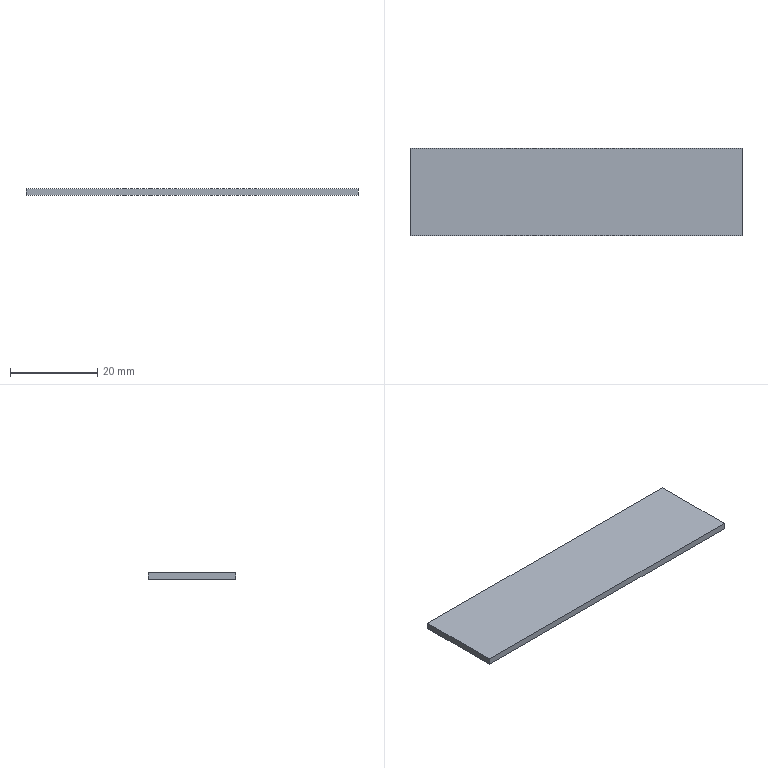Part | STEP file | FHD-021-008-01-C circuit breaker bracket 3 | 1 solid | 6 faces | box 76 x 20 x 1.5 mm | volume 2280 mm3 | plane 6
STEP:
#1=CARTESIAN_POINT('',(0.,0.,0.));
#2=DIRECTION('',(0.,0.,1.));
#3=DIRECTION('',(1.,0.,0.));
#4=AXIS2_PLACEMENT_3D('',#1,#2,#3);
#5=CARTESIAN_POINT('',(-38.,-10.,-1.5));
#6=VERTEX_POINT('',#5);
#7=CARTESIAN_POINT('',(-38.,10.,-1.5));
#8=VERTEX_POINT('',#7);
#9=CARTESIAN_POINT('',(-38.,0.,-1.5));
#10=DIRECTION('',(0.,1.,0.));
#11=VECTOR('',#10,1.);
#12=LINE('',#9,#11);
#13=CARTESIAN_POINT('',(0.,0.,-1.5));
#14=DIRECTION('',(0.,0.,-1.));
#15=DIRECTION('',(-1.,0.,0.));
#16=AXIS2_PLACEMENT_3D('',#13,#14,#15);
#17=PLANE('',#16);
#18=CARTESIAN_POINT('',(38.,0.));
#19=DIRECTION('',(0.,1.));
#20=VECTOR('',#19,1.);
#21=LINE('',#18,#20);
#22=(GEOMETRIC_REPRESENTATION_CONTEXT(2)PARAMETRIC_REPRESENTATION_CONTEXT()REPRESENTATION_CONTEXT('',''));
#23=DEFINITIONAL_REPRESENTATION('',(#21),#22);
#24=PCURVE('',#17,#23);
#25=CARTESIAN_POINT('',(-38.,-10.,-1.5));
#26=DIRECTION('',(-1.,0.,0.));
#27=DIRECTION('',(0.,0.,1.));
#28=AXIS2_PLACEMENT_3D('',#25,#26,#27);
#29=PLANE('',#28);
#30=CARTESIAN_POINT('',(0.,10.));
#31=DIRECTION('',(0.,1.));
#32=VECTOR('',#31,1.);
#33=LINE('',#30,#32);
#34=(GEOMETRIC_REPRESENTATION_CONTEXT(2)PARAMETRIC_REPRESENTATION_CONTEXT()REPRESENTATION_CONTEXT('',''));
#35=DEFINITIONAL_REPRESENTATION('',(#33),#34);
#36=PCURVE('',#29,#35);
#37=SURFACE_CURVE('',#12,(#24,#36),.PCURVE_S1.);
#38=EDGE_CURVE('',#6,#8,#37,.T.);
#39=ORIENTED_EDGE('',*,*,#38,.T.);
#40=CARTESIAN_POINT('',(38.,10.,-1.5));
#41=VERTEX_POINT('',#40);
#42=CARTESIAN_POINT('',(0.,10.,-1.5));
#43=DIRECTION('',(1.,0.,0.));
#44=VECTOR('',#43,1.);
#45=LINE('',#42,#44);
#46=CARTESIAN_POINT('',(0.,10.));
#47=DIRECTION('',(-1.,0.));
#48=VECTOR('',#47,1.);
#49=LINE('',#46,#48);
#50=(GEOMETRIC_REPRESENTATION_CONTEXT(2)PARAMETRIC_REPRESENTATION_CONTEXT()REPRESENTATION_CONTEXT('',''));
#51=DEFINITIONAL_REPRESENTATION('',(#49),#50);
#52=PCURVE('',#17,#51);
#53=CARTESIAN_POINT('',(-38.,10.,-1.5));
#54=DIRECTION('',(0.,1.,0.));
#55=DIRECTION('',(0.,0.,1.));
#56=AXIS2_PLACEMENT_3D('',#53,#54,#55);
#57=PLANE('',#56);
#58=CARTESIAN_POINT('',(0.,38.));
#59=DIRECTION('',(0.,1.));
#60=VECTOR('',#59,1.);
#61=LINE('',#58,#60);
#62=(GEOMETRIC_REPRESENTATION_CONTEXT(2)PARAMETRIC_REPRESENTATION_CONTEXT()REPRESENTATION_CONTEXT('',''));
#63=DEFINITIONAL_REPRESENTATION('',(#61),#62);
#64=PCURVE('',#57,#63);
#65=SURFACE_CURVE('',#45,(#52,#64),.PCURVE_S1.);
#66=EDGE_CURVE('',#8,#41,#65,.T.);
#67=ORIENTED_EDGE('',*,*,#66,.T.);
#68=CARTESIAN_POINT('',(38.,-10.,-1.5));
#69=VERTEX_POINT('',#68);
#70=CARTESIAN_POINT('',(38.,0.,-1.5));
#71=DIRECTION('',(0.,-1.,0.));
#72=VECTOR('',#71,1.);
#73=LINE('',#70,#72);
#74=CARTESIAN_POINT('',(-38.,0.));
#75=DIRECTION('',(0.,-1.));
#76=VECTOR('',#75,1.);
#77=LINE('',#74,#76);
#78=(GEOMETRIC_REPRESENTATION_CONTEXT(2)PARAMETRIC_REPRESENTATION_CONTEXT()REPRESENTATION_CONTEXT('',''));
#79=DEFINITIONAL_REPRESENTATION('',(#77),#78);
#80=PCURVE('',#17,#79);
#81=CARTESIAN_POINT('',(38.,-10.,-1.5));
#82=DIRECTION('',(1.,0.,0.));
#83=DIRECTION('',(0.,0.,-1.));
#84=AXIS2_PLACEMENT_3D('',#81,#82,#83);
#85=PLANE('',#84);
#86=CARTESIAN_POINT('',(0.,10.));
#87=DIRECTION('',(0.,-1.));
#88=VECTOR('',#87,1.);
#89=LINE('',#86,#88);
#90=(GEOMETRIC_REPRESENTATION_CONTEXT(2)PARAMETRIC_REPRESENTATION_CONTEXT()REPRESENTATION_CONTEXT('',''));
#91=DEFINITIONAL_REPRESENTATION('',(#89),#90);
#92=PCURVE('',#85,#91);
#93=SURFACE_CURVE('',#73,(#80,#92),.PCURVE_S1.);
#94=EDGE_CURVE('',#41,#69,#93,.T.);
#95=ORIENTED_EDGE('',*,*,#94,.T.);
#96=CARTESIAN_POINT('',(0.,-10.,-1.5));
#97=DIRECTION('',(-1.,0.,0.));
#98=VECTOR('',#97,1.);
#99=LINE('',#96,#98);
#100=CARTESIAN_POINT('',(0.,-10.));
#101=DIRECTION('',(1.,0.));
#102=VECTOR('',#101,1.);
#103=LINE('',#100,#102);
#104=(GEOMETRIC_REPRESENTATION_CONTEXT(2)PARAMETRIC_REPRESENTATION_CONTEXT()REPRESENTATION_CONTEXT('',''));
#105=DEFINITIONAL_REPRESENTATION('',(#103),#104);
#106=PCURVE('',#17,#105);
#107=CARTESIAN_POINT('',(-38.,-10.,-1.5));
#108=DIRECTION('',(0.,-1.,0.));
#109=DIRECTION('',(0.,0.,-1.));
#110=AXIS2_PLACEMENT_3D('',#107,#108,#109);
#111=PLANE('',#110);
#112=CARTESIAN_POINT('',(0.,38.));
#113=DIRECTION('',(0.,-1.));
#114=VECTOR('',#113,1.);
#115=LINE('',#112,#114);
#116=(GEOMETRIC_REPRESENTATION_CONTEXT(2)PARAMETRIC_REPRESENTATION_CONTEXT()REPRESENTATION_CONTEXT('',''));
#117=DEFINITIONAL_REPRESENTATION('',(#115),#116);
#118=PCURVE('',#111,#117);
#119=SURFACE_CURVE('',#99,(#106,#118),.PCURVE_S1.);
#120=EDGE_CURVE('',#69,#6,#119,.T.);
#121=ORIENTED_EDGE('',*,*,#120,.T.);
#122=EDGE_LOOP('',(#39,#67,#95,#121));
#123=FACE_BOUND('',#122,.T.);
#124=ADVANCED_FACE('',(#123),#17,.T.);
#125=ORIENTED_EDGE('',*,*,#66,.F.);
#126=CARTESIAN_POINT('',(-38.,10.,0.));
#127=VERTEX_POINT('',#126);
#128=CARTESIAN_POINT('',(-38.,10.,-1.5));
#129=DIRECTION('',(0.,0.,1.));
#130=VECTOR('',#129,1.);
#131=LINE('',#128,#130);
#132=CARTESIAN_POINT('',(0.,0.));
#133=DIRECTION('',(1.,0.));
#134=VECTOR('',#133,1.);
#135=LINE('',#132,#134);
#136=(GEOMETRIC_REPRESENTATION_CONTEXT(2)PARAMETRIC_REPRESENTATION_CONTEXT()REPRESENTATION_CONTEXT('',''));
#137=DEFINITIONAL_REPRESENTATION('',(#135),#136);
#138=PCURVE('',#57,#137);
#139=CARTESIAN_POINT('',(0.,20.));
#140=DIRECTION('',(1.,0.));
#141=VECTOR('',#140,1.);
#142=LINE('',#139,#141);
#143=(GEOMETRIC_REPRESENTATION_CONTEXT(2)PARAMETRIC_REPRESENTATION_CONTEXT()REPRESENTATION_CONTEXT('',''));
#144=DEFINITIONAL_REPRESENTATION('',(#142),#143);
#145=PCURVE('',#29,#144);
#146=SURFACE_CURVE('',#131,(#138,#145),.PCURVE_S1.);
#147=EDGE_CURVE('',#8,#127,#146,.T.);
#148=ORIENTED_EDGE('',*,*,#147,.T.);
#149=CARTESIAN_POINT('',(38.,10.,0.));
#150=VERTEX_POINT('',#149);
#151=CARTESIAN_POINT('',(-38.,10.,0.));
#152=DIRECTION('',(1.,0.,0.));
#153=VECTOR('',#152,1.);
#154=LINE('',#151,#153);
#155=CARTESIAN_POINT('',(1.5,0.));
#156=DIRECTION('',(0.,1.));
#157=VECTOR('',#156,1.);
#158=LINE('',#155,#157);
#159=(GEOMETRIC_REPRESENTATION_CONTEXT(2)PARAMETRIC_REPRESENTATION_CONTEXT()REPRESENTATION_CONTEXT('',''));
#160=DEFINITIONAL_REPRESENTATION('',(#158),#159);
#161=PCURVE('',#57,#160);
#162=CARTESIAN_POINT('',(0.,0.,0.));
#163=DIRECTION('',(0.,0.,-1.));
#164=DIRECTION('',(-1.,0.,0.));
#165=AXIS2_PLACEMENT_3D('',#162,#163,#164);
#166=PLANE('',#165);
#167=CARTESIAN_POINT('',(38.,10.));
#168=DIRECTION('',(-1.,0.));
#169=VECTOR('',#168,1.);
#170=LINE('',#167,#169);
#171=(GEOMETRIC_REPRESENTATION_CONTEXT(2)PARAMETRIC_REPRESENTATION_CONTEXT()REPRESENTATION_CONTEXT('',''));
#172=DEFINITIONAL_REPRESENTATION('',(#170),#171);
#173=PCURVE('',#166,#172);
#174=SURFACE_CURVE('',#154,(#161,#173),.PCURVE_S1.);
#175=EDGE_CURVE('',#127,#150,#174,.T.);
#176=ORIENTED_EDGE('',*,*,#175,.T.);
#177=CARTESIAN_POINT('',(38.,10.,-1.5));
#178=DIRECTION('',(0.,0.,-1.));
#179=VECTOR('',#178,1.);
#180=LINE('',#177,#179);
#181=CARTESIAN_POINT('',(0.,76.));
#182=DIRECTION('',(-1.,0.));
#183=VECTOR('',#182,1.);
#184=LINE('',#181,#183);
#185=(GEOMETRIC_REPRESENTATION_CONTEXT(2)PARAMETRIC_REPRESENTATION_CONTEXT()REPRESENTATION_CONTEXT('',''));
#186=DEFINITIONAL_REPRESENTATION('',(#184),#185);
#187=PCURVE('',#57,#186);
#188=CARTESIAN_POINT('',(0.,20.));
#189=DIRECTION('',(1.,0.));
#190=VECTOR('',#189,1.);
#191=LINE('',#188,#190);
#192=(GEOMETRIC_REPRESENTATION_CONTEXT(2)PARAMETRIC_REPRESENTATION_CONTEXT()REPRESENTATION_CONTEXT('',''));
#193=DEFINITIONAL_REPRESENTATION('',(#191),#192);
#194=PCURVE('',#85,#193);
#195=SURFACE_CURVE('',#180,(#187,#194),.PCURVE_S1.);
#196=EDGE_CURVE('',#150,#41,#195,.T.);
#197=ORIENTED_EDGE('',*,*,#196,.T.);
#198=EDGE_LOOP('',(#125,#148,#176,#197));
#199=FACE_BOUND('',#198,.T.);
#200=ADVANCED_FACE('',(#199),#57,.T.);
#201=ORIENTED_EDGE('',*,*,#38,.F.);
#202=CARTESIAN_POINT('',(-38.,-10.,0.));
#203=VERTEX_POINT('',#202);
#204=CARTESIAN_POINT('',(-38.,-10.,-1.5));
#205=DIRECTION('',(0.,0.,1.));
#206=VECTOR('',#205,1.);
#207=LINE('',#204,#206);
#208=CARTESIAN_POINT('',(0.,0.));
#209=DIRECTION('',(1.,0.));
#210=VECTOR('',#209,1.);
#211=LINE('',#208,#210);
#212=(GEOMETRIC_REPRESENTATION_CONTEXT(2)PARAMETRIC_REPRESENTATION_CONTEXT()REPRESENTATION_CONTEXT('',''));
#213=DEFINITIONAL_REPRESENTATION('',(#211),#212);
#214=PCURVE('',#29,#213);
#215=CARTESIAN_POINT('',(0.,0.));
#216=DIRECTION('',(-1.,0.));
#217=VECTOR('',#216,1.);
#218=LINE('',#215,#217);
#219=(GEOMETRIC_REPRESENTATION_CONTEXT(2)PARAMETRIC_REPRESENTATION_CONTEXT()REPRESENTATION_CONTEXT('',''));
#220=DEFINITIONAL_REPRESENTATION('',(#218),#219);
#221=PCURVE('',#111,#220);
#222=SURFACE_CURVE('',#207,(#214,#221),.PCURVE_S1.);
#223=EDGE_CURVE('',#6,#203,#222,.T.);
#224=ORIENTED_EDGE('',*,*,#223,.T.);
#225=CARTESIAN_POINT('',(-38.,-10.,0.));
#226=DIRECTION('',(0.,1.,0.));
#227=VECTOR('',#226,1.);
#228=LINE('',#225,#227);
#229=CARTESIAN_POINT('',(1.5,0.));
#230=DIRECTION('',(0.,1.));
#231=VECTOR('',#230,1.);
#232=LINE('',#229,#231);
#233=(GEOMETRIC_REPRESENTATION_CONTEXT(2)PARAMETRIC_REPRESENTATION_CONTEXT()REPRESENTATION_CONTEXT('',''));
#234=DEFINITIONAL_REPRESENTATION('',(#232),#233);
#235=PCURVE('',#29,#234);
#236=CARTESIAN_POINT('',(38.,-10.));
#237=DIRECTION('',(0.,1.));
#238=VECTOR('',#237,1.);
#239=LINE('',#236,#238);
#240=(GEOMETRIC_REPRESENTATION_CONTEXT(2)PARAMETRIC_REPRESENTATION_CONTEXT()REPRESENTATION_CONTEXT('',''));
#241=DEFINITIONAL_REPRESENTATION('',(#239),#240);
#242=PCURVE('',#166,#241);
#243=SURFACE_CURVE('',#228,(#235,#242),.PCURVE_S1.);
#244=EDGE_CURVE('',#203,#127,#243,.T.);
#245=ORIENTED_EDGE('',*,*,#244,.T.);
#246=ORIENTED_EDGE('',*,*,#147,.F.);
#247=EDGE_LOOP('',(#201,#224,#245,#246));
#248=FACE_BOUND('',#247,.T.);
#249=ADVANCED_FACE('',(#248),#29,.T.);
#250=ORIENTED_EDGE('',*,*,#120,.F.);
#251=CARTESIAN_POINT('',(38.,-10.,0.));
#252=VERTEX_POINT('',#251);
#253=CARTESIAN_POINT('',(38.,-10.,-1.5));
#254=DIRECTION('',(0.,0.,1.));
#255=VECTOR('',#254,1.);
#256=LINE('',#253,#255);
#257=CARTESIAN_POINT('',(0.,76.));
#258=DIRECTION('',(-1.,0.));
#259=VECTOR('',#258,1.);
#260=LINE('',#257,#259);
#261=(GEOMETRIC_REPRESENTATION_CONTEXT(2)PARAMETRIC_REPRESENTATION_CONTEXT()REPRESENTATION_CONTEXT('',''));
#262=DEFINITIONAL_REPRESENTATION('',(#260),#261);
#263=PCURVE('',#111,#262);
#264=CARTESIAN_POINT('',(0.,0.));
#265=DIRECTION('',(-1.,0.));
#266=VECTOR('',#265,1.);
#267=LINE('',#264,#266);
#268=(GEOMETRIC_REPRESENTATION_CONTEXT(2)PARAMETRIC_REPRESENTATION_CONTEXT()REPRESENTATION_CONTEXT('',''));
#269=DEFINITIONAL_REPRESENTATION('',(#267),#268);
#270=PCURVE('',#85,#269);
#271=SURFACE_CURVE('',#256,(#263,#270),.PCURVE_S1.);
#272=EDGE_CURVE('',#69,#252,#271,.T.);
#273=ORIENTED_EDGE('',*,*,#272,.T.);
#274=CARTESIAN_POINT('',(-38.,-10.,0.));
#275=DIRECTION('',(-1.,0.,0.));
#276=VECTOR('',#275,1.);
#277=LINE('',#274,#276);
#278=CARTESIAN_POINT('',(-1.5,0.));
#279=DIRECTION('',(0.,-1.));
#280=VECTOR('',#279,1.);
#281=LINE('',#278,#280);
#282=(GEOMETRIC_REPRESENTATION_CONTEXT(2)PARAMETRIC_REPRESENTATION_CONTEXT()REPRESENTATION_CONTEXT('',''));
#283=DEFINITIONAL_REPRESENTATION('',(#281),#282);
#284=PCURVE('',#111,#283);
#285=CARTESIAN_POINT('',(38.,-10.));
#286=DIRECTION('',(1.,0.));
#287=VECTOR('',#286,1.);
#288=LINE('',#285,#287);
#289=(GEOMETRIC_REPRESENTATION_CONTEXT(2)PARAMETRIC_REPRESENTATION_CONTEXT()REPRESENTATION_CONTEXT('',''));
#290=DEFINITIONAL_REPRESENTATION('',(#288),#289);
#291=PCURVE('',#166,#290);
#292=SURFACE_CURVE('',#277,(#284,#291),.PCURVE_S1.);
#293=EDGE_CURVE('',#252,#203,#292,.T.);
#294=ORIENTED_EDGE('',*,*,#293,.T.);
#295=ORIENTED_EDGE('',*,*,#223,.F.);
#296=EDGE_LOOP('',(#250,#273,#294,#295));
#297=FACE_BOUND('',#296,.T.);
#298=ADVANCED_FACE('',(#297),#111,.T.);
#299=ORIENTED_EDGE('',*,*,#94,.F.);
#300=ORIENTED_EDGE('',*,*,#196,.F.);
#301=CARTESIAN_POINT('',(38.,-10.,0.));
#302=DIRECTION('',(0.,-1.,0.));
#303=VECTOR('',#302,1.);
#304=LINE('',#301,#303);
#305=CARTESIAN_POINT('',(-1.5,0.));
#306=DIRECTION('',(0.,-1.));
#307=VECTOR('',#306,1.);
#308=LINE('',#305,#307);
#309=(GEOMETRIC_REPRESENTATION_CONTEXT(2)PARAMETRIC_REPRESENTATION_CONTEXT()REPRESENTATION_CONTEXT('',''));
#310=DEFINITIONAL_REPRESENTATION('',(#308),#309);
#311=PCURVE('',#85,#310);
#312=CARTESIAN_POINT('',(-38.,-10.));
#313=DIRECTION('',(0.,-1.));
#314=VECTOR('',#313,1.);
#315=LINE('',#312,#314);
#316=(GEOMETRIC_REPRESENTATION_CONTEXT(2)PARAMETRIC_REPRESENTATION_CONTEXT()REPRESENTATION_CONTEXT('',''));
#317=DEFINITIONAL_REPRESENTATION('',(#315),#316);
#318=PCURVE('',#166,#317);
#319=SURFACE_CURVE('',#304,(#311,#318),.PCURVE_S1.);
#320=EDGE_CURVE('',#150,#252,#319,.T.);
#321=ORIENTED_EDGE('',*,*,#320,.T.);
#322=ORIENTED_EDGE('',*,*,#272,.F.);
#323=EDGE_LOOP('',(#299,#300,#321,#322));
#324=FACE_BOUND('',#323,.T.);
#325=ADVANCED_FACE('',(#324),#85,.T.);
#326=ORIENTED_EDGE('',*,*,#175,.F.);
#327=ORIENTED_EDGE('',*,*,#244,.F.);
#328=ORIENTED_EDGE('',*,*,#293,.F.);
#329=ORIENTED_EDGE('',*,*,#320,.F.);
#330=EDGE_LOOP('',(#326,#327,#328,#329));
#331=FACE_BOUND('',#330,.T.);
#332=ADVANCED_FACE('',(#331),#166,.F.);
#333=CLOSED_SHELL('',(#124,#200,#249,#298,#325,#332));
#334=MANIFOLD_SOLID_BREP('',#333);
#335=(LENGTH_UNIT()NAMED_UNIT(*)SI_UNIT(.MILLI.,.METRE.));
#336=UNCERTAINTY_MEASURE_WITH_UNIT(LENGTH_MEASURE(0.0000001),#335,'','');
#337=(NAMED_UNIT(*)PLANE_ANGLE_UNIT()SI_UNIT($,.RADIAN.));
#338=(NAMED_UNIT(*)SI_UNIT($,.STERADIAN.)SOLID_ANGLE_UNIT());
#339=(GEOMETRIC_REPRESENTATION_CONTEXT(3)GLOBAL_UNCERTAINTY_ASSIGNED_CONTEXT((#336))GLOBAL_UNIT_ASSIGNED_CONTEXT((#335,#337,#338))REPRESENTATION_CONTEXT('',''));
#340=ADVANCED_BREP_SHAPE_REPRESENTATION('',(#4,#334),#339);